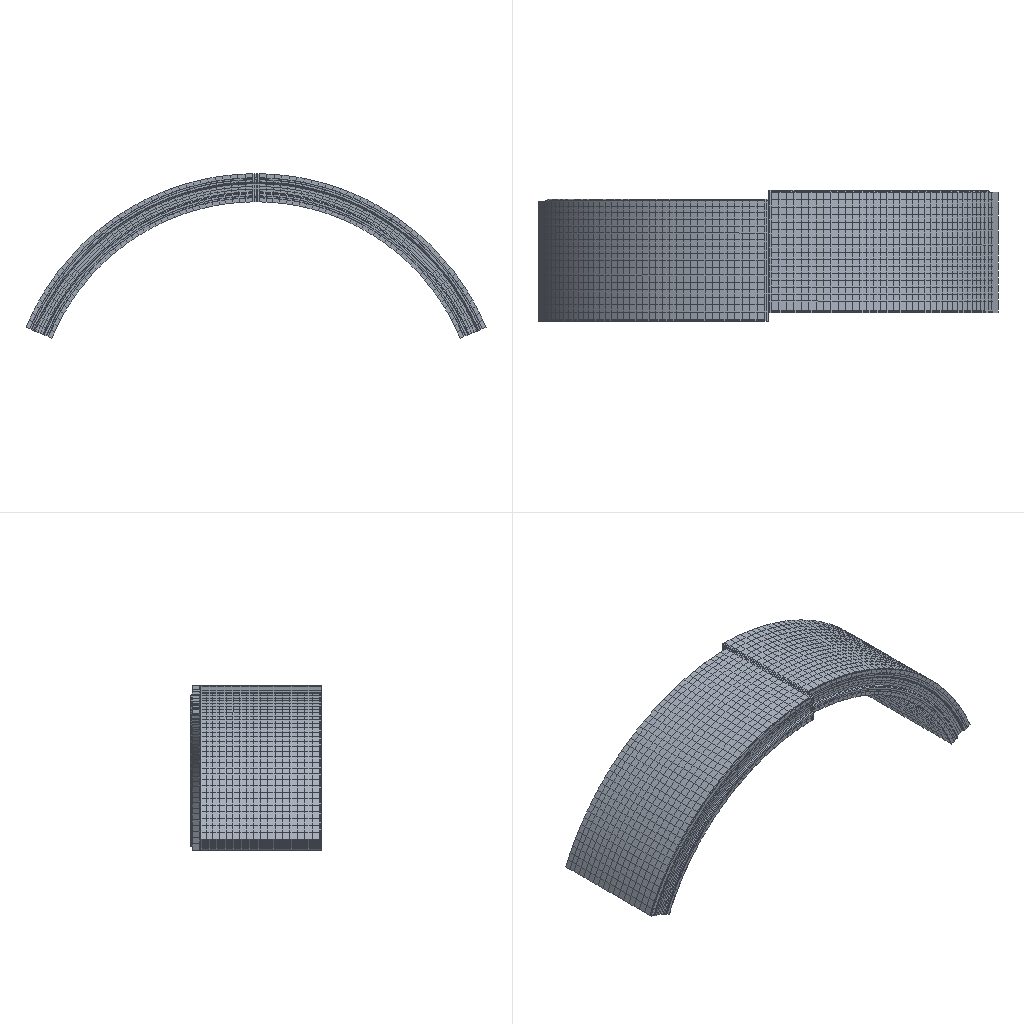Simulation study | abaqus
Set-up summary:
category,name,step,type,value,unit,region
solver,abaqus
solver,version,,,Abaqus/Explicit 2020
units,not stated in the deck,,not stated
analysis,deck,,transient,transient
load_step,Step-1,Step-1,transient
load_step,requested,,,1
mesh,nodes,,,38262
mesh,elements,,,31810
element_type,C3D8R,,solid,31810
load,load commands in deck,,count,2
bc,support commands in deck,,count,16
material,C50,,in results
material,Q345,,in results
check,setup vs results,,match,"per instance, exact: element labels, types and connectivity; labels of the nodes the elements use; coordinates of those nodes at SINGLE_PRECISION in 8 of 8 instance(s)"
Abaqus input file, long lists of numbers shortened:
*Heading
** Job name: Job-1 Model name: Model-1
** Generated by: Abaqus/CAE 2020
*Preprint, echo=NO, model=NO, history=NO, contact=NO
**
** PARTS
**
*Part, name=work-1
*Node
      1,  -41.448,   606.14,  -122.805
      2,  -1556.986,   606.14,  -594.805
** (14922 more lines like these left out)
*Element, type=C3D8R
 1,  394, 3833, 3851,  393,    1,  321,  356,    4
 2, 3833, 3834, 3852, 3851,  321,  322,  355,  356
** (13072 more lines like these left out)
*Nset, nset=Set-1, generate
     1,  14924,      1
*Elset, elset=Set-1, generate
     1,  13074,      1
** Section: con
*Solid Section, elset=Set-1, material=c50
,
*End Part
**
*Part, name=work-2
*Node
      1,   41.448,  -240.005,  -122.805
      2,          2.5,  -238.058,       -122.5
** (14184 more lines like these left out)
*Element, type=C3D8R
1,  328, 3777, 3780,  327,    1,  321,  322,    4
2, 3777,  334,  333, 3780,  321,    2,    3,  322
** (12392 more lines like these left out)
*Nset, nset=Set-1, generate
     1,  14186,      1
*Elset, elset=Set-1, generate
     1,  12394,      1
** Section: con
*Solid Section, elset=Set-1, material=c50
,
*End Part
**
*Part, name=work-3
*Node
      1,  -55.206,   456.828,  -20.246
      2,  -55.456,    456.84,  -25.24
** (1306 more lines like these left out)
*Element, type=C3D8R
 1, 110, 116, 493, 463,   1,   2,  67,  86
 2, 463, 493, 494, 464,  86,  67,  68,  85
** (889 more lines like these left out)
*Nset, nset=Set-1, generate
    1,  1308,     1
*Elset, elset=Set-1, generate
   1,  891,    1
** Section: q345
*Solid Section, elset=Set-1, material=q345
,
*End Part
**
*Part, name=work-4
*Node
      1,  -55.207,    456.828,   20.282
      2,  -54.955,   456.815,   15.252
** (2238 more lines like these left out)
*Element, type=C3D8R
 1,  82,  75,   2,   1, 683, 742, 111,  96
 2,  81,  76,  75,  82, 684, 741, 742, 683
** (1588 more lines like these left out)
*Nset, nset=Set-2, generate
    1,  2240,     1
*Elset, elset=Set-2, generate
    1,  1590,     1
** Section: q345
*Solid Section, elset=Set-2, material=q345
,
*End Part
**
*Part, name=work-5
*Node
      1,   21.972,   560.969,           0.
      2,   21.972,   560.969,          -5.
** (1474 more lines like these left out)
*Element, type=C3D8R
 1, 112, 116, 495, 465,   1,   2,  67,  86
 2, 465, 495, 496, 466,  86,  67,  68,  85
** (1032 more lines like these left out)
*Nset, nset=Set-1, generate
    1,  1476,     1
*Elset, elset=Set-1, generate
    1,  1034,     1
** Section: q345
*Solid Section, elset=Set-1, material=q345
,
*End Part
**
*Part, name=work-6
*Node
      1,   55.206,  -348.828,  -20.246
      2,   60.599,  -240.962,  -20.246
** (1306 more lines like these left out)
*Element, type=C3D8R
 1, 114, 469, 499, 109,   1,  69,  88,   4
 2, 469, 470, 500, 499,  69,  70,  87,  88
** (867 more lines like these left out)
*Nset, nset=Set-1, generate
    1,  1308,     1
*Elset, elset=Set-1, generate
   1,  869,    1
** Section: q345
*Solid Section, elset=Set-1, material=q345
,
*End Part
**
*Part, name=work-7
*Node
      1,   60.349,  -240.95,   15.252
      2,   60.599,  -240.962,   20.246
** (1306 more lines like these left out)
*Element, type=C3D8R
 1, 112, 116, 493, 463,   1,   2,  67,  86
 2, 463, 493, 494, 464,  86,  67,  68,  85
** (889 more lines like these left out)
*Nset, nset=Set-1, generate
    1,  1308,     1
*Elset, elset=Set-1, generate
   1,  891,    1
** Section: q345
*Solid Section, elset=Set-1, material=q345
,
*End Part
**
*Part, name=work-8
*Node
      1,  -21.972,  -452.969,           5.
      2,  -21.972,  -452.969,           0.
** (1510 more lines like these left out)
*Element, type=C3D8R
 1, 116, 120, 515, 485,   1,   2,  71,  90
 2, 485, 515, 516, 486,  90,  71,  72,  89
** (1065 more lines like these left out)
*Nset, nset=Set-1, generate
    1,  1512,     1
*Elset, elset=Set-1, generate
    1,  1067,     1
** Section: q345
*Solid Section, elset=Set-1, material=q345
,
*End Part
**
**
** ASSEMBLY
**
*Assembly, name=Assembly
**
*Instance, name=work-1-1, part=work-1
*End Instance
**
*Instance, name=work-2-1, part=work-2
*End Instance
**
*Instance, name=work-3-1, part=work-3
*End Instance
**
*Instance, name=work-4-1, part=work-4
*End Instance
**
*Instance, name=work-5-1, part=work-5
*End Instance
**
*Instance, name=work-6-1, part=work-6
*End Instance
**
*Instance, name=work-7-1, part=work-7
*End Instance
**
*Instance, name=work-8-1, part=work-8
*End Instance
**
*Nset, nset=Set-1, instance=work-2-1
   257,   258,   259,   260,   261,   262,   267,   268,   269,   270,   271,   272,   273,   274,   275,   276
   279,   280,   281,   282,   283,   284,   285,   286,   287,   288,   289,   290,   291,   292,   293,   294
** (72 more lines like these left out)
*Elset, elset=Set-1, instance=work-2-1
  6437,  6438,  6439,  6440,  6441,  6442,  6443,  6444,  6445,  6446,  6447,  6448,  6449,  6450,  6451,  6452
  6453,  6454,  6455,  6456,  6457,  6458,  6459,  6460,  6461,  6462,  6463,  6464,  6465,  6466,  6467,  6468
** (67 more lines like these left out)
*Nset, nset=Set-2, instance=work-1-1
    51,    52,    53,    54,    55,    56,    57,    58,    59,    60,    61,    62,    63,    64,    66,    67
   103,   104,   105,   106,   107,   108,   109,   110,   111,   112,   113,   114,   155,   156,   157,   158
** (21 more lines like these left out)
*Elset, elset=Set-2, instance=work-1-1
   571,   590,   609,   628,   647,   666,   685,   704,   723,   742,   761,   780,   799,   818,   837,   856
   875,   894,   931,   950,  1079,  1098,  1117,  1136,  1155,  1174,  1193,  1212,  1231,  1250,  1269,  1270
** (19 more lines like these left out)
*Nset, nset=Set-3, instance=work-2-1
   257,   258,   259,   260,   261,   262,   263,   264,   265,   266,   267,   268,   269,   270,   271,   272
   273,   274,   275,   276,   277,   278,   279,   280,   281,   282,   283,   284,   285,   286,   287,   288
** (75 more lines like these left out)
*Elset, elset=Set-3, instance=work-2-1
  6437,  6438,  6439,  6440,  6441,  6442,  6443,  6444,  6445,  6446,  6447,  6448,  6449,  6450,  6451,  6452
  6453,  6454,  6455,  6456,  6457,  6458,  6459,  6460,  6461,  6462,  6463,  6464,  6465,  6466,  6467,  6468
** (71 more lines like these left out)
*Nset, nset=Set-4, instance=work-1-1
     1,     4,     7,     8,     9,    12,    13,    16,    17,    20,    21,    24,    26,    27,    28,    29
    32,    33,    35,    36,    40,    41,    44,    45,    48,    49,    69,    70,    71,    72,    73,    74
** (67 more lines like these left out)
*Elset, elset=Set-4, instance=work-1-1
     1,    20,    39,    58,    77,    96,   115,   134,   153,   172,   191,   210,   283,   284,   285,   340
   341,   342,   361,   380,   399,   418,   437,   456,   475,   494,   513,   532,   551,   570,   951,   970
** (59 more lines like these left out)
*Nset, nset=Set-5, instance=work-1-1
    51,    52,    53,    54,    55,    56,    57,    58,    59,    60,    61,    62,    63,    64,    66,    67
   103,   104,   105,   106,   107,   108,   109,   110,   111,   112,   113,   114,   155,   156,   157,   158
** (21 more lines like these left out)
*Elset, elset=Set-5, instance=work-1-1
   571,   590,   609,   628,   647,   666,   685,   704,   723,   742,   761,   780,   799,   818,   837,   856
   875,   894,   931,   950,  1079,  1098,  1117,  1136,  1155,  1174,  1193,  1212,  1231,  1250,  1269,  1270
** (19 more lines like these left out)
*End Assembly
*Amplitude, name=Amp-1
             0.,              0.,            0.01,              1.
**
** MATERIALS
**
*Material, name=c50
*Density
 2.5e-09,
*Elastic
34500., 0.2
*Concrete Damaged Plasticity
40.,     0.1,    1.16, 0.6667,   0.005
*Concrete Compression Hardening
 23.098,          0.
 25.521,    5.24e-05
 27.759,    7.55e-05
 29.794,  0.0001046
 31.609, 0.00014
 33.194, 0.000182
 34.544, 0.0002309
 35.658, 0.0002866
 36.542, 0.000349
 37.205, 0.0004178
 37.658, 0.0004927
 37.917, 0.0005732
     38.,  0.0006588
 35.822,  0.001074
 31.445,  0.001553
  26.942,  0.002036
   23.05,  0.0025
 19.874,  0.002945
   17.32,  0.003371
 15.263,  0.003782
 13.59,   0.004183
 12.215,  0.004575
 11.072,  0.00496
*Concrete Tension Stiffening
  1.265,          0.
  1.421,    8.21e-06
  1.576,    9.22e-06
  1.728,    1.03e-05
  1.876,    1.15e-05
  2.019,    1.28e-05
  2.155,    1.44e-05
  2.282,    1.62e-05
  2.396,    1.84e-05
  2.494,     2.1e-05
   2.571,    2.43e-05
  2.621,    2.83e-05
     2.64,    3.33e-05
  2.362,    6.33e-05
  1.989,    9.61e-05
  1.681,  0.0001269
  1.445, 0.0001557
  1.265, 0.0001829
  1.125, 0.000209
   1.013, 0.0002341
 0.9232, 0.0002587
 0.849, 0.0002828
 0.7869, 0.0003066
*Concrete Compression Damage
        0.,          0.
 0.03364,    5.24e-05
 0.04387,    7.55e-05
 0.05555,  0.0001046
 0.06862, 0.00014
 0.083, 0.000182
 0.09857, 0.0002309
  0.1152, 0.0002866
  0.1327, 0.000349
  0.151, 0.0004178
  0.1699, 0.0004927
  0.1893, 0.0005732
  0.209,  0.0006588
  0.2989,  0.001074
  0.3919,  0.001553
  0.4734,  0.002036
  0.5408,  0.0025
  0.5955,  0.002945
  0.64,  0.003371
  0.6764,  0.003782
  0.7066,   0.004183
  0.732,  0.004575
  0.7535,  0.00496
  0.7719,  0.00534
  0.7879,  0.005716
  0.8018,  0.006088
  0.8141,  0.006458
  0.8249,  0.006825
  0.8346,  0.007191
  0.8433,  0.007555
   0.8511,  0.007918
  0.8582,  0.00828
  0.8647,   0.00864
  0.8706,  0.009
  0.876,  0.009359
  0.881,  0.009718
  0.8856,   0.01008
  0.8899,   0.01043
  0.9072,   0.01222
  0.9198,   0.01399
** (14 more lines like these left out)
*Concrete Tension Damage
        0.,          0.
 0.08689,    8.21e-06
 0.08786,    9.22e-06
 0.08932,    1.03e-05
 0.09143,    1.15e-05
 0.09437,    1.28e-05
 0.09838,    1.44e-05
  0.1037,    1.62e-05
  0.1108,    1.84e-05
  0.1199,     2.1e-05
  0.1316,    2.43e-05
  0.1465,    2.83e-05
  0.1652,    3.33e-05
  0.2791,    6.33e-05
  0.3875,    9.61e-05
  0.4733,  0.0001269
  0.5396, 0.0001557
  0.5914, 0.0001829
  0.6326, 0.000209
   0.6661, 0.0002341
  0.6938, 0.0002587
  0.7171, 0.0002828
  0.7369, 0.0003066
  0.7539, 0.0003301
  0.7687, 0.0003533
  0.7818, 0.0003764
  0.7933, 0.0003994
  0.8036, 0.0004222
  0.8129, 0.000445
  0.8213, 0.0004677
  0.8288, 0.0004903
  0.8358, 0.0005128
  0.8421, 0.0005353
  0.8479, 0.0005577
  0.8533, 0.0005801
  0.8583, 0.0006025
  0.8629, 0.0006248
  0.8672, 0.0006472
  0.885, 0.0007584
  0.8983, 0.0008693
** (14 more lines like these left out)
*Material, name=q345
*Density
 7.85e-09,
*Elastic
210000., 0.3
*Plastic
345.,0.
**
** INTERACTION PROPERTIES
**
*Surface Interaction, name=IntProp-1
*Friction
 0.1,
*Surface Behavior, pressure-overclosure=HARD
**
** INTERACTIONS
**
** Interaction: Int-1
*Contact, op=NEW
*Contact Inclusions, ALL EXTERIOR
*Contact Property Assignment
 ,  , IntProp-1
** ----------------------------------------------------------------
**
** STEP: Step-1
**
*Step, name=Step-1, nlgeom=YES
*Dynamic, Explicit
, 0.01
*Bulk Viscosity
0.06, 1.2
** Mass Scaling: Semi-Automatic
**               Whole Model
*Fixed Mass Scaling, factor=50.
**
** BOUNDARY CONDITIONS
**
** Name: BC-1 Type: 位移/转角
*Boundary, amplitude=Amp-1
Set-3, 1, 1
Set-3, 2, 2, -108.
Set-3, 3, 3
Set-3, 4, 4
Set-3, 5, 5
Set-3, 6, 6
** Name: BC-3 Type: 位移/转角
*Boundary, amplitude=Amp-1
Set-4, 1, 1, 0.001
Set-4, 2, 2
Set-4, 3, 3
Set-4, 4, 4
Set-4, 5, 5
Set-4, 6, 6
** Name: BC-4 Type: 位移/转角
*Boundary
Set-5, 2, 2
Set-5, 4, 4
Set-5, 5, 5
Set-5, 6, 6
**
** OUTPUT REQUESTS
**
*Restart, write, number interval=1, time marks=NO
**
** FIELD OUTPUT: F-Output-1
**
*Output, field, number interval=50
*Node Output
A, CF, RF, RM, RT, U, V
*Element Output, directions=YES
DAMAGEC, DAMAGET, E, EVF, LE, MISES, MISESMAX, PE, PEEQ, PEEQMAX, PEEQT, PEEQVAVG, PEMAG, PEVAVG, S, SDEG
SF, SVAVG
*Contact Output
CDISP, CSTRESS
**
** HISTORY OUTPUT: H-Output-1
**
*Output, history, variable=PRESELECT, frequency=1
*End Step
Results summary:
result,step,Step-1,completed,increments=12446 time=0.01/0.01
result,analysis,,,transient
result,last_loadstep,,,1
result,primary field,,,U
result,reaction total,,FX,5934281.831,model units
result,reaction total,,FY,-60930765.423,model units
result,reaction total,,FZ,200599.739,model units